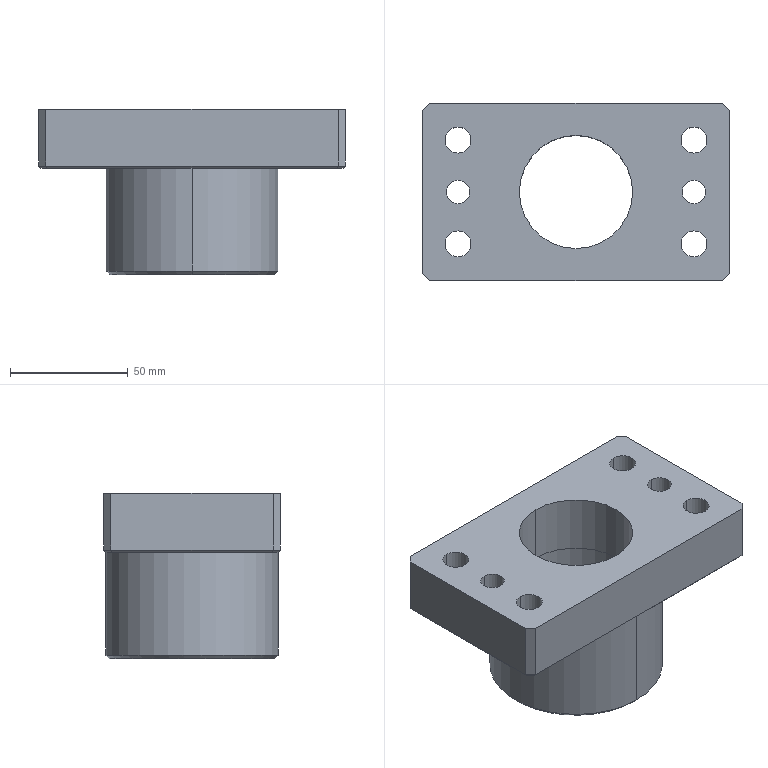Part | STEP file | PN_0058_id1506_x_t | 1 solid | 40 faces | box 130 x 75 x 70 mm | volume 291088 mm3 | plane 20 | cylinder 18 | cone 2 | commonest cylinder face diameters 11 x8 10 x4 48 x4 73 x2
STEP:
#1=CARTESIAN_POINT('',(-260.,-277.5,105.));
#2=VERTEX_POINT('',#1);
#3=CARTESIAN_POINT('',(-260.,-277.5,80.));
#4=VERTEX_POINT('',#3);
#5=CARTESIAN_POINT('',(-260.,-277.5,105.));
#6=DIRECTION('',(0.,0.,-1.));
#7=VECTOR('',#6,1.);
#8=LINE('',#5,#7);
#9=EDGE_CURVE('',#2,#4,#8,.T.);
#10=ORIENTED_EDGE('',*,*,#9,.F.);
#11=CARTESIAN_POINT('',(-260.,-266.5,105.));
#12=VERTEX_POINT('',#11);
#13=CARTESIAN_POINT('',(-260.,-272.,105.));
#14=DIRECTION('',(0.,0.,1.));
#15=DIRECTION('',(0.,-1.,0.));
#16=AXIS2_PLACEMENT_3D('',#13,#14,#15);
#17=CIRCLE('',#16,5.5);
#18=EDGE_CURVE('',#2,#12,#17,.T.);
#19=ORIENTED_EDGE('',*,*,#18,.T.);
#20=CARTESIAN_POINT('',(-260.,-266.5,80.));
#21=VERTEX_POINT('',#20);
#22=CARTESIAN_POINT('',(-260.,-266.5,105.));
#23=DIRECTION('',(0.,0.,1.));
#24=VECTOR('',#23,1.);
#25=LINE('',#22,#24);
#26=EDGE_CURVE('',#21,#12,#25,.T.);
#27=ORIENTED_EDGE('',*,*,#26,.F.);
#28=CARTESIAN_POINT('',(-260.,-272.,80.));
#29=DIRECTION('',(0.,0.,1.));
#30=DIRECTION('',(0.,-1.,0.));
#31=AXIS2_PLACEMENT_3D('',#28,#29,#30);
#32=CIRCLE('',#31,5.5);
#33=EDGE_CURVE('',#4,#21,#32,.T.);
#34=ORIENTED_EDGE('',*,*,#33,.F.);
#35=EDGE_LOOP('',(#10,#19,#27,#34));
#36=FACE_OUTER_BOUND('',#35,.T.);
#37=CARTESIAN_POINT('',(-260.,-272.,105.));
#38=DIRECTION('',(0.,0.,1.));
#39=DIRECTION('',(-1.,0.,0.));
#40=AXIS2_PLACEMENT_3D('',#37,#38,#39);
#41=CYLINDRICAL_SURFACE('',#40,5.5);
#42=ADVANCED_FACE('',(#36),#41,.F.);
#43=ORIENTED_EDGE('',*,*,#26,.T.);
#44=CARTESIAN_POINT('',(-260.,-272.,105.));
#45=DIRECTION('',(0.,0.,1.));
#46=DIRECTION('',(0.,1.,0.));
#47=AXIS2_PLACEMENT_3D('',#44,#45,#46);
#48=CIRCLE('',#47,5.5);
#49=EDGE_CURVE('',#12,#2,#48,.T.);
#50=ORIENTED_EDGE('',*,*,#49,.T.);
#51=ORIENTED_EDGE('',*,*,#9,.T.);
#52=CARTESIAN_POINT('',(-260.,-272.,80.));
#53=DIRECTION('',(0.,0.,1.));
#54=DIRECTION('',(0.,1.,0.));
#55=AXIS2_PLACEMENT_3D('',#52,#53,#54);
#56=CIRCLE('',#55,5.5);
#57=EDGE_CURVE('',#21,#4,#56,.T.);
#58=ORIENTED_EDGE('',*,*,#57,.F.);
#59=EDGE_LOOP('',(#43,#50,#51,#58));
#60=FACE_OUTER_BOUND('',#59,.T.);
#61=CARTESIAN_POINT('',(-260.,-272.,105.));
#62=DIRECTION('',(0.,0.,1.));
#63=DIRECTION('',(1.,0.,0.));
#64=AXIS2_PLACEMENT_3D('',#61,#62,#63);
#65=CYLINDRICAL_SURFACE('',#64,5.5);
#66=ADVANCED_FACE('',(#60),#65,.F.);
#67=CARTESIAN_POINT('',(-260.,-233.5,105.));
#68=VERTEX_POINT('',#67);
#69=CARTESIAN_POINT('',(-260.,-233.5,80.));
#70=VERTEX_POINT('',#69);
#71=CARTESIAN_POINT('',(-260.,-233.5,105.));
#72=DIRECTION('',(0.,0.,-1.));
#73=VECTOR('',#72,1.);
#74=LINE('',#71,#73);
#75=EDGE_CURVE('',#68,#70,#74,.T.);
#76=ORIENTED_EDGE('',*,*,#75,.F.);
#77=CARTESIAN_POINT('',(-260.,-222.5,105.));
#78=VERTEX_POINT('',#77);
#79=CARTESIAN_POINT('',(-260.,-228.,105.));
#80=DIRECTION('',(0.,0.,1.));
#81=DIRECTION('',(0.,-1.,0.));
#82=AXIS2_PLACEMENT_3D('',#79,#80,#81);
#83=CIRCLE('',#82,5.5);
#84=EDGE_CURVE('',#68,#78,#83,.T.);
#85=ORIENTED_EDGE('',*,*,#84,.T.);
#86=CARTESIAN_POINT('',(-260.,-222.5,80.));
#87=VERTEX_POINT('',#86);
#88=CARTESIAN_POINT('',(-260.,-222.5,105.));
#89=DIRECTION('',(0.,0.,1.));
#90=VECTOR('',#89,1.);
#91=LINE('',#88,#90);
#92=EDGE_CURVE('',#87,#78,#91,.T.);
#93=ORIENTED_EDGE('',*,*,#92,.F.);
#94=CARTESIAN_POINT('',(-260.,-228.,80.));
#95=DIRECTION('',(0.,0.,1.));
#96=DIRECTION('',(0.,-1.,0.));
#97=AXIS2_PLACEMENT_3D('',#94,#95,#96);
#98=CIRCLE('',#97,5.5);
#99=EDGE_CURVE('',#70,#87,#98,.T.);
#100=ORIENTED_EDGE('',*,*,#99,.F.);
#101=EDGE_LOOP('',(#76,#85,#93,#100));
#102=FACE_OUTER_BOUND('',#101,.T.);
#103=CARTESIAN_POINT('',(-260.,-228.,105.));
#104=DIRECTION('',(0.,0.,1.));
#105=DIRECTION('',(-1.,0.,0.));
#106=AXIS2_PLACEMENT_3D('',#103,#104,#105);
#107=CYLINDRICAL_SURFACE('',#106,5.5);
#108=ADVANCED_FACE('',(#102),#107,.F.);
#109=ORIENTED_EDGE('',*,*,#92,.T.);
#110=CARTESIAN_POINT('',(-260.,-228.,105.));
#111=DIRECTION('',(0.,0.,1.));
#112=DIRECTION('',(0.,1.,0.));
#113=AXIS2_PLACEMENT_3D('',#110,#111,#112);
#114=CIRCLE('',#113,5.5);
#115=EDGE_CURVE('',#78,#68,#114,.T.);
#116=ORIENTED_EDGE('',*,*,#115,.T.);
#117=ORIENTED_EDGE('',*,*,#75,.T.);
#118=CARTESIAN_POINT('',(-260.,-228.,80.));
#119=DIRECTION('',(0.,0.,1.));
#120=DIRECTION('',(0.,1.,0.));
#121=AXIS2_PLACEMENT_3D('',#118,#119,#120);
#122=CIRCLE('',#121,5.5);
#123=EDGE_CURVE('',#87,#70,#122,.T.);
#124=ORIENTED_EDGE('',*,*,#123,.F.);
#125=EDGE_LOOP('',(#109,#116,#117,#124));
#126=FACE_OUTER_BOUND('',#125,.T.);
#127=CARTESIAN_POINT('',(-260.,-228.,105.));
#128=DIRECTION('',(0.,0.,1.));
#129=DIRECTION('',(1.,0.,0.));
#130=AXIS2_PLACEMENT_3D('',#127,#128,#129);
#131=CYLINDRICAL_SURFACE('',#130,5.5);
#132=ADVANCED_FACE('',(#126),#131,.F.);
#133=CARTESIAN_POINT('',(-160.,-233.5,80.));
#134=VERTEX_POINT('',#133);
#135=CARTESIAN_POINT('',(-160.,-233.5,105.));
#136=VERTEX_POINT('',#135);
#137=CARTESIAN_POINT('',(-160.,-233.5,105.));
#138=DIRECTION('',(0.,0.,1.));
#139=VECTOR('',#138,1.);
#140=LINE('',#137,#139);
#141=EDGE_CURVE('',#134,#136,#140,.T.);
#142=ORIENTED_EDGE('',*,*,#141,.T.);
#143=CARTESIAN_POINT('',(-160.,-222.5,105.));
#144=VERTEX_POINT('',#143);
#145=CARTESIAN_POINT('',(-160.,-228.,105.));
#146=DIRECTION('',(0.,0.,1.));
#147=DIRECTION('',(0.,-1.,0.));
#148=AXIS2_PLACEMENT_3D('',#145,#146,#147);
#149=CIRCLE('',#148,5.5);
#150=EDGE_CURVE('',#136,#144,#149,.T.);
#151=ORIENTED_EDGE('',*,*,#150,.T.);
#152=CARTESIAN_POINT('',(-160.,-222.5,80.));
#153=VERTEX_POINT('',#152);
#154=CARTESIAN_POINT('',(-160.,-222.5,105.));
#155=DIRECTION('',(0.,0.,-1.));
#156=VECTOR('',#155,1.);
#157=LINE('',#154,#156);
#158=EDGE_CURVE('',#144,#153,#157,.T.);
#159=ORIENTED_EDGE('',*,*,#158,.T.);
#160=CARTESIAN_POINT('',(-160.,-228.,80.));
#161=DIRECTION('',(0.,0.,1.));
#162=DIRECTION('',(0.,-1.,0.));
#163=AXIS2_PLACEMENT_3D('',#160,#161,#162);
#164=CIRCLE('',#163,5.5);
#165=EDGE_CURVE('',#134,#153,#164,.T.);
#166=ORIENTED_EDGE('',*,*,#165,.F.);
#167=EDGE_LOOP('',(#142,#151,#159,#166));
#168=FACE_OUTER_BOUND('',#167,.T.);
#169=CARTESIAN_POINT('',(-160.,-228.,105.));
#170=DIRECTION('',(0.,0.,1.));
#171=DIRECTION('',(-1.,0.,0.));
#172=AXIS2_PLACEMENT_3D('',#169,#170,#171);
#173=CYLINDRICAL_SURFACE('',#172,5.5);
#174=ADVANCED_FACE('',(#168),#173,.F.);
#175=ORIENTED_EDGE('',*,*,#158,.F.);
#176=CARTESIAN_POINT('',(-160.,-228.,105.));
#177=DIRECTION('',(0.,0.,1.));
#178=DIRECTION('',(0.,1.,0.));
#179=AXIS2_PLACEMENT_3D('',#176,#177,#178);
#180=CIRCLE('',#179,5.5);
#181=EDGE_CURVE('',#144,#136,#180,.T.);
#182=ORIENTED_EDGE('',*,*,#181,.T.);
#183=ORIENTED_EDGE('',*,*,#141,.F.);
#184=CARTESIAN_POINT('',(-160.,-228.,80.));
#185=DIRECTION('',(0.,0.,1.));
#186=DIRECTION('',(0.,1.,0.));
#187=AXIS2_PLACEMENT_3D('',#184,#185,#186);
#188=CIRCLE('',#187,5.5);
#189=EDGE_CURVE('',#153,#134,#188,.T.);
#190=ORIENTED_EDGE('',*,*,#189,.F.);
#191=EDGE_LOOP('',(#175,#182,#183,#190));
#192=FACE_OUTER_BOUND('',#191,.T.);
#193=CARTESIAN_POINT('',(-160.,-228.,105.));
#194=DIRECTION('',(0.,0.,1.));
#195=DIRECTION('',(1.,0.,0.));
#196=AXIS2_PLACEMENT_3D('',#193,#194,#195);
#197=CYLINDRICAL_SURFACE('',#196,5.5);
#198=ADVANCED_FACE('',(#192),#197,.F.);
#199=CARTESIAN_POINT('',(-160.,-277.5,80.));
#200=VERTEX_POINT('',#199);
#201=CARTESIAN_POINT('',(-160.,-277.5,105.));
#202=VERTEX_POINT('',#201);
#203=CARTESIAN_POINT('',(-160.,-277.5,105.));
#204=DIRECTION('',(0.,0.,1.));
#205=VECTOR('',#204,1.);
#206=LINE('',#203,#205);
#207=EDGE_CURVE('',#200,#202,#206,.T.);
#208=ORIENTED_EDGE('',*,*,#207,.T.);
#209=CARTESIAN_POINT('',(-160.,-266.5,105.));
#210=VERTEX_POINT('',#209);
#211=CARTESIAN_POINT('',(-160.,-272.,105.));
#212=DIRECTION('',(0.,0.,1.));
#213=DIRECTION('',(0.,-1.,0.));
#214=AXIS2_PLACEMENT_3D('',#211,#212,#213);
#215=CIRCLE('',#214,5.5);
#216=EDGE_CURVE('',#202,#210,#215,.T.);
#217=ORIENTED_EDGE('',*,*,#216,.T.);
#218=CARTESIAN_POINT('',(-160.,-266.5,80.));
#219=VERTEX_POINT('',#218);
#220=CARTESIAN_POINT('',(-160.,-266.5,105.));
#221=DIRECTION('',(0.,0.,-1.));
#222=VECTOR('',#221,1.);
#223=LINE('',#220,#222);
#224=EDGE_CURVE('',#210,#219,#223,.T.);
#225=ORIENTED_EDGE('',*,*,#224,.T.);
#226=CARTESIAN_POINT('',(-160.,-272.,80.));
#227=DIRECTION('',(0.,0.,1.));
#228=DIRECTION('',(0.,-1.,0.));
#229=AXIS2_PLACEMENT_3D('',#226,#227,#228);
#230=CIRCLE('',#229,5.5);
#231=EDGE_CURVE('',#200,#219,#230,.T.);
#232=ORIENTED_EDGE('',*,*,#231,.F.);
#233=EDGE_LOOP('',(#208,#217,#225,#232));
#234=FACE_OUTER_BOUND('',#233,.T.);
#235=CARTESIAN_POINT('',(-160.,-272.,105.));
#236=DIRECTION('',(0.,0.,1.));
#237=DIRECTION('',(-1.,0.,0.));
#238=AXIS2_PLACEMENT_3D('',#235,#236,#237);
#239=CYLINDRICAL_SURFACE('',#238,5.5);
#240=ADVANCED_FACE('',(#234),#239,.F.);
#241=ORIENTED_EDGE('',*,*,#224,.F.);
#242=CARTESIAN_POINT('',(-160.,-272.,105.));
#243=DIRECTION('',(0.,0.,1.));
#244=DIRECTION('',(0.,1.,0.));
#245=AXIS2_PLACEMENT_3D('',#242,#243,#244);
#246=CIRCLE('',#245,5.5);
#247=EDGE_CURVE('',#210,#202,#246,.T.);
#248=ORIENTED_EDGE('',*,*,#247,.T.);
#249=ORIENTED_EDGE('',*,*,#207,.F.);
#250=CARTESIAN_POINT('',(-160.,-272.,80.));
#251=DIRECTION('',(0.,0.,1.));
#252=DIRECTION('',(0.,1.,0.));
#253=AXIS2_PLACEMENT_3D('',#250,#251,#252);
#254=CIRCLE('',#253,5.5);
#255=EDGE_CURVE('',#219,#200,#254,.T.);
#256=ORIENTED_EDGE('',*,*,#255,.F.);
#257=EDGE_LOOP('',(#241,#248,#249,#256));
#258=FACE_OUTER_BOUND('',#257,.T.);
#259=CARTESIAN_POINT('',(-160.,-272.,105.));
#260=DIRECTION('',(0.,0.,1.));
#261=DIRECTION('',(1.,0.,0.));
#262=AXIS2_PLACEMENT_3D('',#259,#260,#261);
#263=CYLINDRICAL_SURFACE('',#262,5.5);
#264=ADVANCED_FACE('',(#258),#263,.F.);
#265=CARTESIAN_POINT('',(-210.,-274.,105.));
#266=VERTEX_POINT('',#265);
#267=CARTESIAN_POINT('',(-210.,-274.,80.));
#268=VERTEX_POINT('',#267);
#269=CARTESIAN_POINT('',(-210.,-274.,105.));
#270=DIRECTION('',(0.,0.,-1.));
#271=VECTOR('',#270,1.);
#272=LINE('',#269,#271);
#273=EDGE_CURVE('',#266,#268,#272,.T.);
#274=ORIENTED_EDGE('',*,*,#273,.F.);
#275=CARTESIAN_POINT('',(-210.,-226.,105.));
#276=VERTEX_POINT('',#275);
#277=CARTESIAN_POINT('',(-210.,-250.,105.));
#278=DIRECTION('',(0.,0.,1.));
#279=DIRECTION('',(0.,-1.,0.));
#280=AXIS2_PLACEMENT_3D('',#277,#278,#279);
#281=CIRCLE('',#280,24.);
#282=EDGE_CURVE('',#266,#276,#281,.T.);
#283=ORIENTED_EDGE('',*,*,#282,.T.);
#284=CARTESIAN_POINT('',(-210.,-226.,80.));
#285=VERTEX_POINT('',#284);
#286=CARTESIAN_POINT('',(-210.,-226.,105.));
#287=DIRECTION('',(0.,0.,1.));
#288=VECTOR('',#287,1.);
#289=LINE('',#286,#288);
#290=EDGE_CURVE('',#285,#276,#289,.T.);
#291=ORIENTED_EDGE('',*,*,#290,.F.);
#292=CARTESIAN_POINT('',(-210.,-250.,80.));
#293=DIRECTION('',(0.,0.,1.));
#294=DIRECTION('',(0.,-1.,0.));
#295=AXIS2_PLACEMENT_3D('',#292,#293,#294);
#296=CIRCLE('',#295,24.);
#297=EDGE_CURVE('',#268,#285,#296,.T.);
#298=ORIENTED_EDGE('',*,*,#297,.F.);
#299=EDGE_LOOP('',(#274,#283,#291,#298));
#300=FACE_OUTER_BOUND('',#299,.T.);
#301=CARTESIAN_POINT('',(-210.,-250.,105.));
#302=DIRECTION('',(0.,0.,1.));
#303=DIRECTION('',(-1.,0.008727,0.));
#304=AXIS2_PLACEMENT_3D('',#301,#302,#303);
#305=CYLINDRICAL_SURFACE('',#304,24.);
#306=ADVANCED_FACE('',(#300),#305,.F.);
#307=ORIENTED_EDGE('',*,*,#290,.T.);
#308=CARTESIAN_POINT('',(-210.,-250.,105.));
#309=DIRECTION('',(0.,0.,1.));
#310=DIRECTION('',(0.,1.,0.));
#311=AXIS2_PLACEMENT_3D('',#308,#309,#310);
#312=CIRCLE('',#311,24.);
#313=EDGE_CURVE('',#276,#266,#312,.T.);
#314=ORIENTED_EDGE('',*,*,#313,.T.);
#315=ORIENTED_EDGE('',*,*,#273,.T.);
#316=CARTESIAN_POINT('',(-210.,-250.,80.));
#317=DIRECTION('',(0.,0.,1.));
#318=DIRECTION('',(0.,1.,0.));
#319=AXIS2_PLACEMENT_3D('',#316,#317,#318);
#320=CIRCLE('',#319,24.);
#321=EDGE_CURVE('',#285,#268,#320,.T.);
#322=ORIENTED_EDGE('',*,*,#321,.F.);
#323=EDGE_LOOP('',(#307,#314,#315,#322));
#324=FACE_OUTER_BOUND('',#323,.T.);
#325=CARTESIAN_POINT('',(-210.,-250.,105.));
#326=DIRECTION('',(0.,0.,1.));
#327=DIRECTION('',(1.,0.,0.));
#328=AXIS2_PLACEMENT_3D('',#325,#326,#327);
#329=CYLINDRICAL_SURFACE('',#328,24.);
#330=ADVANCED_FACE('',(#324),#329,.F.);
#331=ORIENTED_EDGE('',*,*,#297,.T.);
#332=CARTESIAN_POINT('',(-210.,-226.,35.));
#333=VERTEX_POINT('',#332);
#334=CARTESIAN_POINT('',(-210.,-226.,80.));
#335=DIRECTION('',(0.,0.,-1.));
#336=VECTOR('',#335,1.);
#337=LINE('',#334,#336);
#338=EDGE_CURVE('',#285,#333,#337,.T.);
#339=ORIENTED_EDGE('',*,*,#338,.T.);
#340=CARTESIAN_POINT('',(-210.,-274.,35.));
#341=VERTEX_POINT('',#340);
#342=CARTESIAN_POINT('',(-210.,-250.,35.));
#343=DIRECTION('',(0.,0.,1.));
#344=DIRECTION('',(0.,-1.,0.));
#345=AXIS2_PLACEMENT_3D('',#342,#343,#344);
#346=CIRCLE('',#345,24.);
#347=EDGE_CURVE('',#341,#333,#346,.T.);
#348=ORIENTED_EDGE('',*,*,#347,.F.);
#349=CARTESIAN_POINT('',(-210.,-274.,80.));
#350=DIRECTION('',(0.,0.,1.));
#351=VECTOR('',#350,1.);
#352=LINE('',#349,#351);
#353=EDGE_CURVE('',#341,#268,#352,.T.);
#354=ORIENTED_EDGE('',*,*,#353,.T.);
#355=EDGE_LOOP('',(#331,#339,#348,#354));
#356=FACE_OUTER_BOUND('',#355,.T.);
#357=CARTESIAN_POINT('',(-210.,-250.,105.));
#358=DIRECTION('',(0.,0.,1.));
#359=DIRECTION('',(-1.,0.008727,0.));
#360=AXIS2_PLACEMENT_3D('',#357,#358,#359);
#361=CYLINDRICAL_SURFACE('',#360,24.);
#362=ADVANCED_FACE('',(#356),#361,.F.);
#363=ORIENTED_EDGE('',*,*,#321,.T.);
#364=ORIENTED_EDGE('',*,*,#353,.F.);
#365=CARTESIAN_POINT('',(-210.,-250.,35.));
#366=DIRECTION('',(0.,0.,1.));
#367=DIRECTION('',(0.,1.,0.));
#368=AXIS2_PLACEMENT_3D('',#365,#366,#367);
#369=CIRCLE('',#368,24.);
#370=EDGE_CURVE('',#333,#341,#369,.T.);
#371=ORIENTED_EDGE('',*,*,#370,.F.);
#372=ORIENTED_EDGE('',*,*,#338,.F.);
#373=EDGE_LOOP('',(#363,#364,#371,#372));
#374=FACE_OUTER_BOUND('',#373,.T.);
#375=CARTESIAN_POINT('',(-210.,-250.,105.));
#376=DIRECTION('',(0.,0.,1.));
#377=DIRECTION('',(1.,0.,0.));
#378=AXIS2_PLACEMENT_3D('',#375,#376,#377);
#379=CYLINDRICAL_SURFACE('',#378,24.);
#380=ADVANCED_FACE('',(#374),#379,.F.);
#381=CARTESIAN_POINT('',(-260.,-245.,105.));
#382=VERTEX_POINT('',#381);
#383=CARTESIAN_POINT('',(-260.,-245.,80.));
#384=VERTEX_POINT('',#383);
#385=CARTESIAN_POINT('',(-260.,-245.,105.));
#386=DIRECTION('',(0.,0.,-1.));
#387=VECTOR('',#386,1.);
#388=LINE('',#385,#387);
#389=EDGE_CURVE('',#382,#384,#388,.T.);
#390=ORIENTED_EDGE('',*,*,#389,.F.);
#391=CARTESIAN_POINT('',(-260.,-255.,105.));
#392=VERTEX_POINT('',#391);
#393=CARTESIAN_POINT('',(-260.,-250.,105.));
#394=DIRECTION('',(0.,0.,1.));
#395=DIRECTION('',(0.,1.,0.));
#396=AXIS2_PLACEMENT_3D('',#393,#394,#395);
#397=CIRCLE('',#396,5.);
#398=EDGE_CURVE('',#382,#392,#397,.T.);
#399=ORIENTED_EDGE('',*,*,#398,.T.);
#400=CARTESIAN_POINT('',(-260.,-255.,80.));
#401=VERTEX_POINT('',#400);
#402=CARTESIAN_POINT('',(-260.,-255.,105.));
#403=DIRECTION('',(0.,0.,1.));
#404=VECTOR('',#403,1.);
#405=LINE('',#402,#404);
#406=EDGE_CURVE('',#401,#392,#405,.T.);
#407=ORIENTED_EDGE('',*,*,#406,.F.);
#408=CARTESIAN_POINT('',(-260.,-250.,80.));
#409=DIRECTION('',(0.,0.,-1.));
#410=DIRECTION('',(0.,-1.,0.));
#411=AXIS2_PLACEMENT_3D('',#408,#409,#410);
#412=CIRCLE('',#411,5.);
#413=EDGE_CURVE('',#401,#384,#412,.T.);
#414=ORIENTED_EDGE('',*,*,#413,.T.);
#415=EDGE_LOOP('',(#390,#399,#407,#414));
#416=FACE_OUTER_BOUND('',#415,.T.);
#417=CARTESIAN_POINT('',(-260.,-250.,105.));
#418=DIRECTION('',(0.,0.,1.));
#419=DIRECTION('',(1.,0.,0.));
#420=AXIS2_PLACEMENT_3D('',#417,#418,#419);
#421=CYLINDRICAL_SURFACE('',#420,5.);
#422=ADVANCED_FACE('',(#416),#421,.F.);
#423=ORIENTED_EDGE('',*,*,#389,.T.);
#424=CARTESIAN_POINT('',(-260.,-250.,80.));
#425=DIRECTION('',(0.,0.,-1.));
#426=DIRECTION('',(0.,1.,0.));
#427=AXIS2_PLACEMENT_3D('',#424,#425,#426);
#428=CIRCLE('',#427,5.);
#429=EDGE_CURVE('',#384,#401,#428,.T.);
#430=ORIENTED_EDGE('',*,*,#429,.T.);
#431=ORIENTED_EDGE('',*,*,#406,.T.);
#432=CARTESIAN_POINT('',(-260.,-250.,105.));
#433=DIRECTION('',(0.,0.,1.));
#434=DIRECTION('',(0.,-1.,0.));
#435=AXIS2_PLACEMENT_3D('',#432,#433,#434);
#436=CIRCLE('',#435,5.);
#437=EDGE_CURVE('',#392,#382,#436,.T.);
#438=ORIENTED_EDGE('',*,*,#437,.T.);
#439=EDGE_LOOP('',(#423,#430,#431,#438));
#440=FACE_OUTER_BOUND('',#439,.T.);
#441=CARTESIAN_POINT('',(-260.,-250.,105.));
#442=DIRECTION('',(0.,0.,1.));
#443=DIRECTION('',(-1.,0.,0.));
#444=AXIS2_PLACEMENT_3D('',#441,#442,#443);
#445=CYLINDRICAL_SURFACE('',#444,5.);
#446=ADVANCED_FACE('',(#440),#445,.F.);
#447=CARTESIAN_POINT('',(-160.,-245.,105.));
#448=VERTEX_POINT('',#447);
#449=CARTESIAN_POINT('',(-160.,-245.,80.));
#450=VERTEX_POINT('',#449);
#451=CARTESIAN_POINT('',(-160.,-245.,105.));
#452=DIRECTION('',(0.,0.,-1.));
#453=VECTOR('',#452,1.);
#454=LINE('',#451,#453);
#455=EDGE_CURVE('',#448,#450,#454,.T.);
#456=ORIENTED_EDGE('',*,*,#455,.F.);
#457=CARTESIAN_POINT('',(-160.,-255.,105.));
#458=VERTEX_POINT('',#457);
#459=CARTESIAN_POINT('',(-160.,-250.,105.));
#460=DIRECTION('',(0.,0.,1.));
#461=DIRECTION('',(0.,1.,0.));
#462=AXIS2_PLACEMENT_3D('',#459,#460,#461);
#463=CIRCLE('',#462,5.);
#464=EDGE_CURVE('',#448,#458,#463,.T.);
#465=ORIENTED_EDGE('',*,*,#464,.T.);
#466=CARTESIAN_POINT('',(-160.,-255.,80.));
#467=VERTEX_POINT('',#466);
#468=CARTESIAN_POINT('',(-160.,-255.,105.));
#469=DIRECTION('',(0.,0.,1.));
#470=VECTOR('',#469,1.);
#471=LINE('',#468,#470);
#472=EDGE_CURVE('',#467,#458,#471,.T.);
#473=ORIENTED_EDGE('',*,*,#472,.F.);
#474=CARTESIAN_POINT('',(-160.,-250.,80.));
#475=DIRECTION('',(0.,0.,-1.));
#476=DIRECTION('',(0.,-1.,0.));
#477=AXIS2_PLACEMENT_3D('',#474,#475,#476);
#478=CIRCLE('',#477,5.);
#479=EDGE_CURVE('',#467,#450,#478,.T.);
#480=ORIENTED_EDGE('',*,*,#479,.T.);
#481=EDGE_LOOP('',(#456,#465,#473,#480));
#482=FACE_OUTER_BOUND('',#481,.T.);
#483=CARTESIAN_POINT('',(-160.,-250.,105.));
#484=DIRECTION('',(0.,0.,1.));
#485=DIRECTION('',(1.,0.,0.));
#486=AXIS2_PLACEMENT_3D('',#483,#484,#485);
#487=CYLINDRICAL_SURFACE('',#486,5.);
#488=ADVANCED_FACE('',(#482),#487,.F.);
#489=ORIENTED_EDGE('',*,*,#455,.T.);
#490=CARTESIAN_POINT('',(-160.,-250.,80.));
#491=DIRECTION('',(0.,0.,-1.));
#492=DIRECTION('',(0.,1.,0.));
#493=AXIS2_PLACEMENT_3D('',#490,#491,#492);
#494=CIRCLE('',#493,5.);
#495=EDGE_CURVE('',#450,#467,#494,.T.);
#496=ORIENTED_EDGE('',*,*,#495,.T.);
#497=ORIENTED_EDGE('',*,*,#472,.T.);
#498=CARTESIAN_POINT('',(-160.,-250.,105.));
#499=DIRECTION('',(0.,0.,1.));
#500=DIRECTION('',(0.,-1.,0.));
#501=AXIS2_PLACEMENT_3D('',#498,#499,#500);
#502=CIRCLE('',#501,5.);
#503=EDGE_CURVE('',#458,#448,#502,.T.);
#504=ORIENTED_EDGE('',*,*,#503,.T.);
#505=EDGE_LOOP('',(#489,#496,#497,#504));
#506=FACE_OUTER_BOUND('',#505,.T.);
#507=CARTESIAN_POINT('',(-160.,-250.,105.));
#508=DIRECTION('',(0.,0.,1.));
#509=DIRECTION('',(-1.,0.,0.));
#510=AXIS2_PLACEMENT_3D('',#507,#508,#509);
#511=CYLINDRICAL_SURFACE('',#510,5.);
#512=ADVANCED_FACE('',(#506),#511,.F.);
#513=CARTESIAN_POINT('',(-148.,-212.5,105.));
#514=VERTEX_POINT('',#513);
#515=CARTESIAN_POINT('',(-145.,-215.5,105.));
#516=VERTEX_POINT('',#515);
#517=CARTESIAN_POINT('',(-148.,-212.5,105.));
#518=DIRECTION('',(0.7071,-0.7071,0.));
#519=VECTOR('',#518,1.);
#520=LINE('',#517,#519);
#521=EDGE_CURVE('',#514,#516,#520,.T.);
#522=ORIENTED_EDGE('',*,*,#521,.F.);
#523=CARTESIAN_POINT('',(-272.,-212.5,105.));
#524=VERTEX_POINT('',#523);
#525=CARTESIAN_POINT('',(-272.,-212.5,105.));
#526=DIRECTION('',(1.,0.,0.));
#527=VECTOR('',#526,1.);
#528=LINE('',#525,#527);
#529=EDGE_CURVE('',#524,#514,#528,.T.);
#530=ORIENTED_EDGE('',*,*,#529,.F.);
#531=CARTESIAN_POINT('',(-275.,-215.5,105.));
#532=VERTEX_POINT('',#531);
#533=CARTESIAN_POINT('',(-275.,-215.5,105.));
#534=DIRECTION('',(0.7071,0.7071,0.));
#535=VECTOR('',#534,1.);
#536=LINE('',#533,#535);
#537=EDGE_CURVE('',#532,#524,#536,.T.);
#538=ORIENTED_EDGE('',*,*,#537,.F.);
#539=CARTESIAN_POINT('',(-275.,-284.5,105.));
#540=VERTEX_POINT('',#539);
#541=CARTESIAN_POINT('',(-275.,-284.5,105.));
#542=DIRECTION('',(0.,1.,0.));
#543=VECTOR('',#542,1.);
#544=LINE('',#541,#543);
#545=EDGE_CURVE('',#540,#532,#544,.T.);
#546=ORIENTED_EDGE('',*,*,#545,.F.);
#547=CARTESIAN_POINT('',(-272.,-287.5,105.));
#548=VERTEX_POINT('',#547);
#549=CARTESIAN_POINT('',(-272.,-287.5,105.));
#550=DIRECTION('',(-0.7071,0.7071,0.));
#551=VECTOR('',#550,1.);
#552=LINE('',#549,#551);
#553=EDGE_CURVE('',#548,#540,#552,.T.);
#554=ORIENTED_EDGE('',*,*,#553,.F.);
#555=CARTESIAN_POINT('',(-148.,-287.5,105.));
#556=VERTEX_POINT('',#555);
#557=CARTESIAN_POINT('',(-148.,-287.5,105.));
#558=DIRECTION('',(-1.,0.,0.));
#559=VECTOR('',#558,1.);
#560=LINE('',#557,#559);
#561=EDGE_CURVE('',#556,#548,#560,.T.);
#562=ORIENTED_EDGE('',*,*,#561,.F.);
#563=CARTESIAN_POINT('',(-145.,-284.5,105.));
#564=VERTEX_POINT('',#563);
#565=CARTESIAN_POINT('',(-145.,-284.5,105.));
#566=DIRECTION('',(-0.7071,-0.7071,0.));
#567=VECTOR('',#566,1.);
#568=LINE('',#565,#567);
#569=EDGE_CURVE('',#564,#556,#568,.T.);
#570=ORIENTED_EDGE('',*,*,#569,.F.);
#571=CARTESIAN_POINT('',(-145.,-215.5,105.));
#572=DIRECTION('',(0.,-1.,0.));
#573=VECTOR('',#572,1.);
#574=LINE('',#571,#573);
#575=EDGE_CURVE('',#516,#564,#574,.T.);
#576=ORIENTED_EDGE('',*,*,#575,.F.);
#577=EDGE_LOOP('',(#522,#530,#538,#546,#554,#562,#570,#576));
#578=FACE_BOUND('',#577,.T.);
#579=ORIENTED_EDGE('',*,*,#503,.F.);
#580=ORIENTED_EDGE('',*,*,#464,.F.);
#581=EDGE_LOOP('',(#579,#580));
#582=FACE_BOUND('',#581,.T.);
#583=ORIENTED_EDGE('',*,*,#437,.F.);
#584=ORIENTED_EDGE('',*,*,#398,.F.);
#585=EDGE_LOOP('',(#583,#584));
#586=FACE_BOUND('',#585,.T.);
#587=ORIENTED_EDGE('',*,*,#18,.F.);
#588=ORIENTED_EDGE('',*,*,#49,.F.);
#589=EDGE_LOOP('',(#587,#588));
#590=FACE_BOUND('',#589,.T.);
#591=ORIENTED_EDGE('',*,*,#84,.F.);
#592=ORIENTED_EDGE('',*,*,#115,.F.);
#593=EDGE_LOOP('',(#591,#592));
#594=FACE_BOUND('',#593,.T.);
#595=ORIENTED_EDGE('',*,*,#150,.F.);
#596=ORIENTED_EDGE('',*,*,#181,.F.);
#597=EDGE_LOOP('',(#595,#596));
#598=FACE_BOUND('',#597,.T.);
#599=ORIENTED_EDGE('',*,*,#216,.F.);
#600=ORIENTED_EDGE('',*,*,#247,.F.);
#601=EDGE_LOOP('',(#599,#600));
#602=FACE_BOUND('',#601,.T.);
#603=ORIENTED_EDGE('',*,*,#282,.F.);
#604=ORIENTED_EDGE('',*,*,#313,.F.);
#605=EDGE_LOOP('',(#603,#604));
#606=FACE_BOUND('',#605,.T.);
#607=CARTESIAN_POINT('',(-285.,-295.,105.));
#608=DIRECTION('',(0.,0.,1.));
#609=DIRECTION('',(1.,0.,0.));
#610=AXIS2_PLACEMENT_3D('',#607,#608,#609);
#611=PLANE('',#610);
#612=ADVANCED_FACE('',(#578,#582,#586,#590,#594,#598,#602,#606),#611,.T.);
#613=CARTESIAN_POINT('',(-210.,-286.5,36.5));
#614=VERTEX_POINT('',#613);
#615=CARTESIAN_POINT('',(-210.,-213.5,36.5));
#616=VERTEX_POINT('',#615);
#617=CARTESIAN_POINT('',(-210.,-250.,36.5));
#618=DIRECTION('',(0.,0.,-1.));
#619=DIRECTION('',(0.,-1.,0.));
#620=AXIS2_PLACEMENT_3D('',#617,#618,#619);
#621=CIRCLE('',#620,36.5);
#622=EDGE_CURVE('',#614,#616,#621,.T.);
#623=ORIENTED_EDGE('',*,*,#622,.F.);
#624=CARTESIAN_POINT('',(-210.,-286.5,80.));
#625=VERTEX_POINT('',#624);
#626=CARTESIAN_POINT('',(-210.,-286.5,80.));
#627=DIRECTION('',(0.,0.,1.));
#628=VECTOR('',#627,1.);
#629=LINE('',#626,#628);
#630=EDGE_CURVE('',#614,#625,#629,.T.);
#631=ORIENTED_EDGE('',*,*,#630,.T.);
#632=CARTESIAN_POINT('',(-210.,-213.5,80.));
#633=VERTEX_POINT('',#632);
#634=CARTESIAN_POINT('',(-210.,-250.,80.));
#635=DIRECTION('',(0.,0.,-1.));
#636=DIRECTION('',(0.,-1.,0.));
#637=AXIS2_PLACEMENT_3D('',#634,#635,#636);
#638=CIRCLE('',#637,36.5);
#639=EDGE_CURVE('',#625,#633,#638,.T.);
#640=ORIENTED_EDGE('',*,*,#639,.T.);
#641=CARTESIAN_POINT('',(-210.,-213.5,80.));
#642=DIRECTION('',(0.,0.,-1.));
#643=VECTOR('',#642,1.);
#644=LINE('',#641,#643);
#645=EDGE_CURVE('',#633,#616,#644,.T.);
#646=ORIENTED_EDGE('',*,*,#645,.T.);
#647=EDGE_LOOP('',(#623,#631,#640,#646));
#648=FACE_OUTER_BOUND('',#647,.T.);
#649=CARTESIAN_POINT('',(-210.,-250.,105.));
#650=DIRECTION('',(0.,0.,1.));
#651=DIRECTION('',(1.,0.,0.));
#652=AXIS2_PLACEMENT_3D('',#649,#650,#651);
#653=CYLINDRICAL_SURFACE('',#652,36.5);
#654=ADVANCED_FACE('',(#648),#653,.T.);
#655=CARTESIAN_POINT('',(-210.,-250.,36.5));
#656=DIRECTION('',(0.,0.,-1.));
#657=DIRECTION('',(0.,1.,0.));
#658=AXIS2_PLACEMENT_3D('',#655,#656,#657);
#659=CIRCLE('',#658,36.5);
#660=EDGE_CURVE('',#616,#614,#659,.T.);
#661=ORIENTED_EDGE('',*,*,#660,.F.);
#662=ORIENTED_EDGE('',*,*,#645,.F.);
#663=CARTESIAN_POINT('',(-210.,-250.,80.));
#664=DIRECTION('',(0.,0.,-1.));
#665=DIRECTION('',(0.,1.,0.));
#666=AXIS2_PLACEMENT_3D('',#663,#664,#665);
#667=CIRCLE('',#666,36.5);
#668=EDGE_CURVE('',#633,#625,#667,.T.);
#669=ORIENTED_EDGE('',*,*,#668,.T.);
#670=ORIENTED_EDGE('',*,*,#630,.F.);
#671=EDGE_LOOP('',(#661,#662,#669,#670));
#672=FACE_OUTER_BOUND('',#671,.T.);
#673=CARTESIAN_POINT('',(-210.,-250.,105.));
#674=DIRECTION('',(0.,0.,1.));
#675=DIRECTION('',(-1.,0.,0.));
#676=AXIS2_PLACEMENT_3D('',#673,#674,#675);
#677=CYLINDRICAL_SURFACE('',#676,36.5);
#678=ADVANCED_FACE('',(#672),#677,.T.);
#679=CARTESIAN_POINT('',(-210.,-215.,35.));
#680=VERTEX_POINT('',#679);
#681=CARTESIAN_POINT('',(-210.,-285.,35.));
#682=VERTEX_POINT('',#681);
#683=CARTESIAN_POINT('',(-210.,-250.,35.));
#684=DIRECTION('',(0.,0.,1.));
#685=DIRECTION('',(0.,1.,0.));
#686=AXIS2_PLACEMENT_3D('',#683,#684,#685);
#687=CIRCLE('',#686,35.);
#688=EDGE_CURVE('',#680,#682,#687,.T.);
#689=ORIENTED_EDGE('',*,*,#688,.F.);
#690=CARTESIAN_POINT('',(-210.,-250.,35.));
#691=DIRECTION('',(0.,0.,1.));
#692=DIRECTION('',(0.,-1.,0.));
#693=AXIS2_PLACEMENT_3D('',#690,#691,#692);
#694=CIRCLE('',#693,35.);
#695=EDGE_CURVE('',#682,#680,#694,.T.);
#696=ORIENTED_EDGE('',*,*,#695,.F.);
#697=EDGE_LOOP('',(#689,#696));
#698=FACE_BOUND('',#697,.T.);
#699=ORIENTED_EDGE('',*,*,#347,.T.);
#700=ORIENTED_EDGE('',*,*,#370,.T.);
#701=EDGE_LOOP('',(#699,#700));
#702=FACE_BOUND('',#701,.T.);
#703=CARTESIAN_POINT('',(-168.,-208.,35.));
#704=DIRECTION('',(0.,0.,-1.));
#705=DIRECTION('',(0.,-1.,0.));
#706=AXIS2_PLACEMENT_3D('',#703,#704,#705);
#707=PLANE('',#706);
#708=ADVANCED_FACE('',(#698,#702),#707,.T.);
#709=CARTESIAN_POINT('',(-210.,-213.5,36.5));
#710=DIRECTION('',(0.,0.7071,0.7071));
#711=VECTOR('',#710,1.);
#712=LINE('',#709,#711);
#713=EDGE_CURVE('',#680,#616,#712,.T.);
#714=ORIENTED_EDGE('',*,*,#713,.F.);
#715=ORIENTED_EDGE('',*,*,#688,.T.);
#716=CARTESIAN_POINT('',(-210.,-286.5,36.5));
#717=DIRECTION('',(0.,0.7071,-0.7071));
#718=VECTOR('',#717,1.);
#719=LINE('',#716,#718);
#720=EDGE_CURVE('',#614,#682,#719,.T.);
#721=ORIENTED_EDGE('',*,*,#720,.F.);
#722=ORIENTED_EDGE('',*,*,#622,.T.);
#723=EDGE_LOOP('',(#714,#715,#721,#722));
#724=FACE_OUTER_BOUND('',#723,.T.);
#725=CARTESIAN_POINT('',(-210.,-250.,36.5));
#726=DIRECTION('',(0.,0.,1.));
#727=DIRECTION('',(0.9998,0.01745,0.));
#728=AXIS2_PLACEMENT_3D('',#725,#726,#727);
#729=CONICAL_SURFACE('',#728,36.5,45.);
#730=ADVANCED_FACE('',(#724),#729,.T.);
#731=ORIENTED_EDGE('',*,*,#713,.T.);
#732=ORIENTED_EDGE('',*,*,#660,.T.);
#733=ORIENTED_EDGE('',*,*,#720,.T.);
#734=ORIENTED_EDGE('',*,*,#695,.T.);
#735=EDGE_LOOP('',(#731,#732,#733,#734));
#736=FACE_OUTER_BOUND('',#735,.T.);
#737=CARTESIAN_POINT('',(-210.,-250.,36.5));
#738=DIRECTION('',(0.,0.,1.));
#739=DIRECTION('',(-1.,0.,0.));
#740=AXIS2_PLACEMENT_3D('',#737,#738,#739);
#741=CONICAL_SURFACE('',#740,36.5,45.);
#742=ADVANCED_FACE('',(#736),#741,.T.);
#743=CARTESIAN_POINT('',(-272.,-287.5,81.));
#744=VERTEX_POINT('',#743);
#745=CARTESIAN_POINT('',(-275.,-284.5,81.));
#746=VERTEX_POINT('',#745);
#747=CARTESIAN_POINT('',(-272.,-287.5,81.));
#748=DIRECTION('',(-0.7071,0.7071,0.));
#749=VECTOR('',#748,1.);
#750=LINE('',#747,#749);
#751=EDGE_CURVE('',#744,#746,#750,.T.);
#752=ORIENTED_EDGE('',*,*,#751,.F.);
#753=CARTESIAN_POINT('',(-272.,-287.5,81.));
#754=DIRECTION('',(0.,0.,1.));
#755=VECTOR('',#754,1.);
#756=LINE('',#753,#755);
#757=EDGE_CURVE('',#744,#548,#756,.T.);
#758=ORIENTED_EDGE('',*,*,#757,.T.);
#759=ORIENTED_EDGE('',*,*,#553,.T.);
#760=CARTESIAN_POINT('',(-275.,-284.5,105.));
#761=DIRECTION('',(0.,0.,-1.));
#762=VECTOR('',#761,1.);
#763=LINE('',#760,#762);
#764=EDGE_CURVE('',#540,#746,#763,.T.);
#765=ORIENTED_EDGE('',*,*,#764,.T.);
#766=EDGE_LOOP('',(#752,#758,#759,#765));
#767=FACE_OUTER_BOUND('',#766,.T.);
#768=CARTESIAN_POINT('',(-271.7,-287.8,107.4));
#769=DIRECTION('',(-0.7071,-0.7071,0.));
#770=DIRECTION('',(-0.7071,0.7071,0.));
#771=AXIS2_PLACEMENT_3D('',#768,#769,#770);
#772=PLANE('',#771);
#773=ADVANCED_FACE('',(#767),#772,.T.);
#774=CARTESIAN_POINT('',(-275.,-215.5,81.));
#775=VERTEX_POINT('',#774);
#776=CARTESIAN_POINT('',(-272.,-212.5,81.));
#777=VERTEX_POINT('',#776);
#778=CARTESIAN_POINT('',(-275.,-215.5,81.));
#779=DIRECTION('',(0.7071,0.7071,0.));
#780=VECTOR('',#779,1.);
#781=LINE('',#778,#780);
#782=EDGE_CURVE('',#775,#777,#781,.T.);
#783=ORIENTED_EDGE('',*,*,#782,.F.);
#784=CARTESIAN_POINT('',(-275.,-215.5,81.));
#785=DIRECTION('',(0.,0.,1.));
#786=VECTOR('',#785,1.);
#787=LINE('',#784,#786);
#788=EDGE_CURVE('',#775,#532,#787,.T.);
#789=ORIENTED_EDGE('',*,*,#788,.T.);
#790=ORIENTED_EDGE('',*,*,#537,.T.);
#791=CARTESIAN_POINT('',(-272.,-212.5,105.));
#792=DIRECTION('',(0.,0.,-1.));
#793=VECTOR('',#792,1.);
#794=LINE('',#791,#793);
#795=EDGE_CURVE('',#524,#777,#794,.T.);
#796=ORIENTED_EDGE('',*,*,#795,.T.);
#797=EDGE_LOOP('',(#783,#789,#790,#796));
#798=FACE_OUTER_BOUND('',#797,.T.);
#799=CARTESIAN_POINT('',(-275.3,-215.8,78.6));
#800=DIRECTION('',(-0.7071,0.7071,0.));
#801=DIRECTION('',(0.,0.,1.));
#802=AXIS2_PLACEMENT_3D('',#799,#800,#801);
#803=PLANE('',#802);
#804=ADVANCED_FACE('',(#798),#803,.T.);
#805=CARTESIAN_POINT('',(-148.,-212.5,81.));
#806=VERTEX_POINT('',#805);
#807=CARTESIAN_POINT('',(-145.,-215.5,81.));
#808=VERTEX_POINT('',#807);
#809=CARTESIAN_POINT('',(-148.,-212.5,81.));
#810=DIRECTION('',(0.7071,-0.7071,0.));
#811=VECTOR('',#810,1.);
#812=LINE('',#809,#811);
#813=EDGE_CURVE('',#806,#808,#812,.T.);
#814=ORIENTED_EDGE('',*,*,#813,.F.);
#815=CARTESIAN_POINT('',(-148.,-212.5,81.));
#816=DIRECTION('',(0.,0.,1.));
#817=VECTOR('',#816,1.);
#818=LINE('',#815,#817);
#819=EDGE_CURVE('',#806,#514,#818,.T.);
#820=ORIENTED_EDGE('',*,*,#819,.T.);
#821=ORIENTED_EDGE('',*,*,#521,.T.);
#822=CARTESIAN_POINT('',(-145.,-215.5,105.));
#823=DIRECTION('',(0.,0.,-1.));
#824=VECTOR('',#823,1.);
#825=LINE('',#822,#824);
#826=EDGE_CURVE('',#516,#808,#825,.T.);
#827=ORIENTED_EDGE('',*,*,#826,.T.);
#828=EDGE_LOOP('',(#814,#820,#821,#827));
#829=FACE_OUTER_BOUND('',#828,.T.);
#830=CARTESIAN_POINT('',(-144.7,-215.8,107.4));
#831=DIRECTION('',(0.7071,0.7071,0.));
#832=DIRECTION('',(0.,0.,-1.));
#833=AXIS2_PLACEMENT_3D('',#830,#831,#832);
#834=PLANE('',#833);
#835=ADVANCED_FACE('',(#829),#834,.T.);
#836=CARTESIAN_POINT('',(-145.,-284.5,81.));
#837=VERTEX_POINT('',#836);
#838=CARTESIAN_POINT('',(-148.,-287.5,81.));
#839=VERTEX_POINT('',#838);
#840=CARTESIAN_POINT('',(-145.,-284.5,81.));
#841=DIRECTION('',(-0.7071,-0.7071,0.));
#842=VECTOR('',#841,1.);
#843=LINE('',#840,#842);
#844=EDGE_CURVE('',#837,#839,#843,.T.);
#845=ORIENTED_EDGE('',*,*,#844,.F.);
#846=CARTESIAN_POINT('',(-145.,-284.5,81.));
#847=DIRECTION('',(0.,0.,1.));
#848=VECTOR('',#847,1.);
#849=LINE('',#846,#848);
#850=EDGE_CURVE('',#837,#564,#849,.T.);
#851=ORIENTED_EDGE('',*,*,#850,.T.);
#852=ORIENTED_EDGE('',*,*,#569,.T.);
#853=CARTESIAN_POINT('',(-148.,-287.5,105.));
#854=DIRECTION('',(0.,0.,-1.));
#855=VECTOR('',#854,1.);
#856=LINE('',#853,#855);
#857=EDGE_CURVE('',#556,#839,#856,.T.);
#858=ORIENTED_EDGE('',*,*,#857,.T.);
#859=EDGE_LOOP('',(#845,#851,#852,#858));
#860=FACE_OUTER_BOUND('',#859,.T.);
#861=CARTESIAN_POINT('',(-148.3,-287.8,107.4));
#862=DIRECTION('',(0.7071,-0.7071,0.));
#863=DIRECTION('',(0.,0.,-1.));
#864=AXIS2_PLACEMENT_3D('',#861,#862,#863);
#865=PLANE('',#864);
#866=ADVANCED_FACE('',(#860),#865,.T.);
#867=CARTESIAN_POINT('',(-145.,-215.5,81.));
#868=DIRECTION('',(0.,-1.,0.));
#869=VECTOR('',#868,1.);
#870=LINE('',#867,#869);
#871=EDGE_CURVE('',#808,#837,#870,.T.);
#872=ORIENTED_EDGE('',*,*,#871,.F.);
#873=ORIENTED_EDGE('',*,*,#826,.F.);
#874=ORIENTED_EDGE('',*,*,#575,.T.);
#875=ORIENTED_EDGE('',*,*,#850,.F.);
#876=EDGE_LOOP('',(#872,#873,#874,#875));
#877=FACE_OUTER_BOUND('',#876,.T.);
#878=CARTESIAN_POINT('',(-145.,-291.4,78.6));
#879=DIRECTION('',(1.,0.,0.));
#880=DIRECTION('',(0.,1.,0.));
#881=AXIS2_PLACEMENT_3D('',#878,#879,#880);
#882=PLANE('',#881);
#883=ADVANCED_FACE('',(#877),#882,.T.);
#884=CARTESIAN_POINT('',(-146.,-215.914,80.));
#885=VERTEX_POINT('',#884);
#886=CARTESIAN_POINT('',(-146.,-215.914,80.));
#887=DIRECTION('',(0.6786,0.2811,0.6786));
#888=VECTOR('',#887,1.);
#889=LINE('',#886,#888);
#890=EDGE_CURVE('',#885,#808,#889,.T.);
#891=ORIENTED_EDGE('',*,*,#890,.T.);
#892=ORIENTED_EDGE('',*,*,#871,.T.);
#893=CARTESIAN_POINT('',(-146.,-284.086,80.));
#894=VERTEX_POINT('',#893);
#895=CARTESIAN_POINT('',(-145.,-284.5,81.));
#896=DIRECTION('',(-0.6786,0.2811,-0.6786));
#897=VECTOR('',#896,1.);
#898=LINE('',#895,#897);
#899=EDGE_CURVE('',#837,#894,#898,.T.);
#900=ORIENTED_EDGE('',*,*,#899,.T.);
#901=CARTESIAN_POINT('',(-146.,-284.086,80.));
#902=DIRECTION('',(0.,1.,0.));
#903=VECTOR('',#902,1.);
#904=LINE('',#901,#903);
#905=EDGE_CURVE('',#894,#885,#904,.T.);
#906=ORIENTED_EDGE('',*,*,#905,.T.);
#907=EDGE_LOOP('',(#891,#892,#900,#906));
#908=FACE_OUTER_BOUND('',#907,.T.);
#909=CARTESIAN_POINT('',(-144.9,-208.6,81.1));
#910=DIRECTION('',(0.7071,0.,-0.7071));
#911=DIRECTION('',(0.,-1.,0.));
#912=AXIS2_PLACEMENT_3D('',#909,#910,#911);
#913=PLANE('',#912);
#914=ADVANCED_FACE('',(#908),#913,.T.);
#915=CARTESIAN_POINT('',(-148.414,-213.5,80.));
#916=VERTEX_POINT('',#915);
#917=CARTESIAN_POINT('',(-148.,-212.5,81.));
#918=DIRECTION('',(-0.2811,-0.6786,-0.6786));
#919=VECTOR('',#918,1.);
#920=LINE('',#917,#919);
#921=EDGE_CURVE('',#806,#916,#920,.T.);
#922=ORIENTED_EDGE('',*,*,#921,.F.);
#923=ORIENTED_EDGE('',*,*,#813,.T.);
#924=ORIENTED_EDGE('',*,*,#890,.F.);
#925=CARTESIAN_POINT('',(-146.,-215.914,80.));
#926=DIRECTION('',(-0.7071,0.7071,0.));
#927=VECTOR('',#926,1.);
#928=LINE('',#925,#927);
#929=EDGE_CURVE('',#885,#916,#928,.T.);
#930=ORIENTED_EDGE('',*,*,#929,.T.);
#931=EDGE_LOOP('',(#922,#923,#924,#930));
#932=FACE_OUTER_BOUND('',#931,.T.);
#933=CARTESIAN_POINT('',(-144.659,-213.339,82.769));
#934=DIRECTION('',(0.5,0.5,-0.7071));
#935=DIRECTION('',(0.,-0.8165,-0.5774));
#936=AXIS2_PLACEMENT_3D('',#933,#934,#935);
#937=PLANE('',#936);
#938=ADVANCED_FACE('',(#932),#937,.T.);
#939=CARTESIAN_POINT('',(-272.,-212.5,81.));
#940=DIRECTION('',(1.,0.,0.));
#941=VECTOR('',#940,1.);
#942=LINE('',#939,#941);
#943=EDGE_CURVE('',#777,#806,#942,.T.);
#944=ORIENTED_EDGE('',*,*,#943,.F.);
#945=ORIENTED_EDGE('',*,*,#795,.F.);
#946=ORIENTED_EDGE('',*,*,#529,.T.);
#947=ORIENTED_EDGE('',*,*,#819,.F.);
#948=EDGE_LOOP('',(#944,#945,#946,#947));
#949=FACE_OUTER_BOUND('',#948,.T.);
#950=CARTESIAN_POINT('',(-282.,-212.5,107.4));
#951=DIRECTION('',(0.,1.,0.));
#952=DIRECTION('',(1.,0.,0.));
#953=AXIS2_PLACEMENT_3D('',#950,#951,#952);
#954=PLANE('',#953);
#955=ADVANCED_FACE('',(#949),#954,.T.);
#956=CARTESIAN_POINT('',(-271.586,-213.5,80.));
#957=VERTEX_POINT('',#956);
#958=CARTESIAN_POINT('',(-271.586,-213.5,80.));
#959=DIRECTION('',(-0.2811,0.6786,0.6786));
#960=VECTOR('',#959,1.);
#961=LINE('',#958,#960);
#962=EDGE_CURVE('',#957,#777,#961,.T.);
#963=ORIENTED_EDGE('',*,*,#962,.T.);
#964=ORIENTED_EDGE('',*,*,#943,.T.);
#965=ORIENTED_EDGE('',*,*,#921,.T.);
#966=CARTESIAN_POINT('',(-148.414,-213.5,80.));
#967=DIRECTION('',(-1.,0.,0.));
#968=VECTOR('',#967,1.);
#969=LINE('',#966,#968);
#970=EDGE_CURVE('',#916,#633,#969,.T.);
#971=ORIENTED_EDGE('',*,*,#970,.T.);
#972=CARTESIAN_POINT('',(-210.,-213.5,80.));
#973=DIRECTION('',(-1.,0.,0.));
#974=VECTOR('',#973,1.);
#975=LINE('',#972,#974);
#976=EDGE_CURVE('',#633,#957,#975,.T.);
#977=ORIENTED_EDGE('',*,*,#976,.T.);
#978=EDGE_LOOP('',(#963,#964,#965,#971,#977));
#979=FACE_OUTER_BOUND('',#978,.T.);
#980=CARTESIAN_POINT('',(-138.,-213.6,79.9));
#981=DIRECTION('',(0.,0.7071,-0.7071));
#982=DIRECTION('',(-1.,0.,0.));
#983=AXIS2_PLACEMENT_3D('',#980,#981,#982);
#984=PLANE('',#983);
#985=ADVANCED_FACE('',(#979),#984,.T.);
#986=CARTESIAN_POINT('',(-274.,-215.914,80.));
#987=VERTEX_POINT('',#986);
#988=CARTESIAN_POINT('',(-275.,-215.5,81.));
#989=DIRECTION('',(0.6786,-0.2811,-0.6786));
#990=VECTOR('',#989,1.);
#991=LINE('',#988,#990);
#992=EDGE_CURVE('',#775,#987,#991,.T.);
#993=ORIENTED_EDGE('',*,*,#992,.F.);
#994=ORIENTED_EDGE('',*,*,#782,.T.);
#995=ORIENTED_EDGE('',*,*,#962,.F.);
#996=CARTESIAN_POINT('',(-271.586,-213.5,80.));
#997=DIRECTION('',(-0.7071,-0.7071,0.));
#998=VECTOR('',#997,1.);
#999=LINE('',#996,#998);
#1000=EDGE_CURVE('',#957,#987,#999,.T.);
#1001=ORIENTED_EDGE('',*,*,#1000,.T.);
#1002=EDGE_LOOP('',(#993,#994,#995,#1001));
#1003=FACE_OUTER_BOUND('',#1002,.T.);
#1004=CARTESIAN_POINT('',(-272.23,-216.256,78.507));
#1005=DIRECTION('',(-0.5,0.5,-0.7071));
#1006=DIRECTION('',(-0.8165,0.,0.5774));
#1007=AXIS2_PLACEMENT_3D('',#1004,#1005,#1006);
#1008=PLANE('',#1007);
#1009=ADVANCED_FACE('',(#1003),#1008,.T.);
#1010=CARTESIAN_POINT('',(-275.,-284.5,81.));
#1011=DIRECTION('',(0.,1.,0.));
#1012=VECTOR('',#1011,1.);
#1013=LINE('',#1010,#1012);
#1014=EDGE_CURVE('',#746,#775,#1013,.T.);
#1015=ORIENTED_EDGE('',*,*,#1014,.F.);
#1016=ORIENTED_EDGE('',*,*,#764,.F.);
#1017=ORIENTED_EDGE('',*,*,#545,.T.);
#1018=ORIENTED_EDGE('',*,*,#788,.F.);
#1019=EDGE_LOOP('',(#1015,#1016,#1017,#1018));
#1020=FACE_OUTER_BOUND('',#1019,.T.);
#1021=CARTESIAN_POINT('',(-275.,-291.4,78.6));
#1022=DIRECTION('',(-1.,0.,0.));
#1023=DIRECTION('',(0.,0.,1.));
#1024=AXIS2_PLACEMENT_3D('',#1021,#1022,#1023);
#1025=PLANE('',#1024);
#1026=ADVANCED_FACE('',(#1020),#1025,.T.);
#1027=CARTESIAN_POINT('',(-274.,-284.086,80.));
#1028=VERTEX_POINT('',#1027);
#1029=CARTESIAN_POINT('',(-274.,-284.086,80.));
#1030=DIRECTION('',(-0.6786,-0.2811,0.6786));
#1031=VECTOR('',#1030,1.);
#1032=LINE('',#1029,#1031);
#1033=EDGE_CURVE('',#1028,#746,#1032,.T.);
#1034=ORIENTED_EDGE('',*,*,#1033,.T.);
#1035=ORIENTED_EDGE('',*,*,#1014,.T.);
#1036=ORIENTED_EDGE('',*,*,#992,.T.);
#1037=CARTESIAN_POINT('',(-274.,-215.914,80.));
#1038=DIRECTION('',(0.,-1.,0.));
#1039=VECTOR('',#1038,1.);
#1040=LINE('',#1037,#1039);
#1041=EDGE_CURVE('',#987,#1028,#1040,.T.);
#1042=ORIENTED_EDGE('',*,*,#1041,.T.);
#1043=EDGE_LOOP('',(#1034,#1035,#1036,#1042));
#1044=FACE_OUTER_BOUND('',#1043,.T.);
#1045=CARTESIAN_POINT('',(-273.9,-291.4,79.9));
#1046=DIRECTION('',(-0.7071,0.,-0.7071));
#1047=DIRECTION('',(-0.7071,0.,0.7071));
#1048=AXIS2_PLACEMENT_3D('',#1045,#1046,#1047);
#1049=PLANE('',#1048);
#1050=ADVANCED_FACE('',(#1044),#1049,.T.);
#1051=CARTESIAN_POINT('',(-271.586,-286.5,80.));
#1052=VERTEX_POINT('',#1051);
#1053=CARTESIAN_POINT('',(-272.,-287.5,81.));
#1054=DIRECTION('',(0.2811,0.6786,-0.6786));
#1055=VECTOR('',#1054,1.);
#1056=LINE('',#1053,#1055);
#1057=EDGE_CURVE('',#744,#1052,#1056,.T.);
#1058=ORIENTED_EDGE('',*,*,#1057,.F.);
#1059=ORIENTED_EDGE('',*,*,#751,.T.);
#1060=ORIENTED_EDGE('',*,*,#1033,.F.);
#1061=CARTESIAN_POINT('',(-274.,-284.086,80.));
#1062=DIRECTION('',(0.7071,-0.7071,0.));
#1063=VECTOR('',#1062,1.);
#1064=LINE('',#1061,#1063);
#1065=EDGE_CURVE('',#1028,#1052,#1064,.T.);
#1066=ORIENTED_EDGE('',*,*,#1065,.T.);
#1067=EDGE_LOOP('',(#1058,#1059,#1060,#1066));
#1068=FACE_OUTER_BOUND('',#1067,.T.);
#1069=CARTESIAN_POINT('',(-271.244,-284.73,78.507));
#1070=DIRECTION('',(-0.5,-0.5,-0.7071));
#1071=DIRECTION('',(0.,-0.8165,0.5774));
#1072=AXIS2_PLACEMENT_3D('',#1069,#1070,#1071);
#1073=PLANE('',#1072);
#1074=ADVANCED_FACE('',(#1068),#1073,.T.);
#1075=CARTESIAN_POINT('',(-271.586,-286.5,80.));
#1076=DIRECTION('',(1.,0.,0.));
#1077=VECTOR('',#1076,1.);
#1078=LINE('',#1075,#1077);
#1079=EDGE_CURVE('',#1052,#625,#1078,.T.);
#1080=ORIENTED_EDGE('',*,*,#1079,.F.);
#1081=ORIENTED_EDGE('',*,*,#1065,.F.);
#1082=ORIENTED_EDGE('',*,*,#1041,.F.);
#1083=ORIENTED_EDGE('',*,*,#1000,.F.);
#1084=ORIENTED_EDGE('',*,*,#976,.F.);
#1085=ORIENTED_EDGE('',*,*,#639,.F.);
#1086=EDGE_LOOP('',(#1080,#1081,#1082,#1083,#1084,#1085));
#1087=FACE_BOUND('',#1086,.T.);
#1088=ORIENTED_EDGE('',*,*,#429,.F.);
#1089=ORIENTED_EDGE('',*,*,#413,.F.);
#1090=EDGE_LOOP('',(#1088,#1089));
#1091=FACE_BOUND('',#1090,.T.);
#1092=ORIENTED_EDGE('',*,*,#33,.T.);
#1093=ORIENTED_EDGE('',*,*,#57,.T.);
#1094=EDGE_LOOP('',(#1092,#1093));
#1095=FACE_BOUND('',#1094,.T.);
#1096=ORIENTED_EDGE('',*,*,#99,.T.);
#1097=ORIENTED_EDGE('',*,*,#123,.T.);
#1098=EDGE_LOOP('',(#1096,#1097));
#1099=FACE_BOUND('',#1098,.T.);
#1100=CARTESIAN_POINT('',(-203.6,-206.2,80.));
#1101=DIRECTION('',(0.,0.,-1.));
#1102=DIRECTION('',(0.,-1.,0.));
#1103=AXIS2_PLACEMENT_3D('',#1100,#1101,#1102);
#1104=PLANE('',#1103);
#1105=ADVANCED_FACE('',(#1087,#1091,#1095,#1099),#1104,.T.);
#1106=CARTESIAN_POINT('',(-148.414,-286.5,80.));
#1107=VERTEX_POINT('',#1106);
#1108=CARTESIAN_POINT('',(-210.,-286.5,80.));
#1109=DIRECTION('',(1.,0.,0.));
#1110=VECTOR('',#1109,1.);
#1111=LINE('',#1108,#1110);
#1112=EDGE_CURVE('',#625,#1107,#1111,.T.);
#1113=ORIENTED_EDGE('',*,*,#1112,.F.);
#1114=ORIENTED_EDGE('',*,*,#668,.F.);
#1115=ORIENTED_EDGE('',*,*,#970,.F.);
#1116=ORIENTED_EDGE('',*,*,#929,.F.);
#1117=ORIENTED_EDGE('',*,*,#905,.F.);
#1118=CARTESIAN_POINT('',(-148.414,-286.5,80.));
#1119=DIRECTION('',(0.7071,0.7071,0.));
#1120=VECTOR('',#1119,1.);
#1121=LINE('',#1118,#1120);
#1122=EDGE_CURVE('',#1107,#894,#1121,.T.);
#1123=ORIENTED_EDGE('',*,*,#1122,.F.);
#1124=EDGE_LOOP('',(#1113,#1114,#1115,#1116,#1117,#1123));
#1125=FACE_BOUND('',#1124,.T.);
#1126=ORIENTED_EDGE('',*,*,#495,.F.);
#1127=ORIENTED_EDGE('',*,*,#479,.F.);
#1128=EDGE_LOOP('',(#1126,#1127));
#1129=FACE_BOUND('',#1128,.T.);
#1130=ORIENTED_EDGE('',*,*,#165,.T.);
#1131=ORIENTED_EDGE('',*,*,#189,.T.);
#1132=EDGE_LOOP('',(#1130,#1131));
#1133=FACE_BOUND('',#1132,.T.);
#1134=ORIENTED_EDGE('',*,*,#231,.T.);
#1135=ORIENTED_EDGE('',*,*,#255,.T.);
#1136=EDGE_LOOP('',(#1134,#1135));
#1137=FACE_BOUND('',#1136,.T.);
#1138=CARTESIAN_POINT('',(-139.6,-206.2,80.));
#1139=DIRECTION('',(0.,0.,-1.));
#1140=DIRECTION('',(0.,-1.,0.));
#1141=AXIS2_PLACEMENT_3D('',#1138,#1139,#1140);
#1142=PLANE('',#1141);
#1143=ADVANCED_FACE('',(#1125,#1129,#1133,#1137),#1142,.T.);
#1144=CARTESIAN_POINT('',(-148.414,-286.5,80.));
#1145=DIRECTION('',(0.2811,-0.6786,0.6786));
#1146=VECTOR('',#1145,1.);
#1147=LINE('',#1144,#1146);
#1148=EDGE_CURVE('',#1107,#839,#1147,.T.);
#1149=ORIENTED_EDGE('',*,*,#1148,.F.);
#1150=ORIENTED_EDGE('',*,*,#1122,.T.);
#1151=ORIENTED_EDGE('',*,*,#899,.F.);
#1152=ORIENTED_EDGE('',*,*,#844,.T.);
#1153=EDGE_LOOP('',(#1149,#1150,#1151,#1152));
#1154=FACE_OUTER_BOUND('',#1153,.T.);
#1155=CARTESIAN_POINT('',(-144.659,-283.364,80.438));
#1156=DIRECTION('',(0.5,-0.5,-0.7071));
#1157=DIRECTION('',(0.,-0.8165,0.5774));
#1158=AXIS2_PLACEMENT_3D('',#1155,#1156,#1157);
#1159=PLANE('',#1158);
#1160=ADVANCED_FACE('',(#1154),#1159,.T.);
#1161=CARTESIAN_POINT('',(-148.,-287.5,81.));
#1162=DIRECTION('',(-1.,0.,0.));
#1163=VECTOR('',#1162,1.);
#1164=LINE('',#1161,#1163);
#1165=EDGE_CURVE('',#839,#744,#1164,.T.);
#1166=ORIENTED_EDGE('',*,*,#1165,.F.);
#1167=ORIENTED_EDGE('',*,*,#857,.F.);
#1168=ORIENTED_EDGE('',*,*,#561,.T.);
#1169=ORIENTED_EDGE('',*,*,#757,.F.);
#1170=EDGE_LOOP('',(#1166,#1167,#1168,#1169));
#1171=FACE_OUTER_BOUND('',#1170,.T.);
#1172=CARTESIAN_POINT('',(-282.,-287.5,107.4));
#1173=DIRECTION('',(0.,-1.,0.));
#1174=DIRECTION('',(0.,0.,-1.));
#1175=AXIS2_PLACEMENT_3D('',#1172,#1173,#1174);
#1176=PLANE('',#1175);
#1177=ADVANCED_FACE('',(#1171),#1176,.T.);
#1178=ORIENTED_EDGE('',*,*,#1148,.T.);
#1179=ORIENTED_EDGE('',*,*,#1165,.T.);
#1180=ORIENTED_EDGE('',*,*,#1057,.T.);
#1181=ORIENTED_EDGE('',*,*,#1079,.T.);
#1182=ORIENTED_EDGE('',*,*,#1112,.T.);
#1183=EDGE_LOOP('',(#1178,#1179,#1180,#1181,#1182));
#1184=FACE_OUTER_BOUND('',#1183,.T.);
#1185=CARTESIAN_POINT('',(-138.,-286.4,79.9));
#1186=DIRECTION('',(0.,-0.7071,-0.7071));
#1187=DIRECTION('',(0.,-0.7071,0.7071));
#1188=AXIS2_PLACEMENT_3D('',#1185,#1186,#1187);
#1189=PLANE('',#1188);
#1190=ADVANCED_FACE('',(#1184),#1189,.T.);
#1191=CLOSED_SHELL('',(#42,#66,#108,#132,#174,#198,#240,#264,#306,#330,#362,#380,#422,#446,#488,#512,#612,#654,#678,#708,#730,#742,#773,#804,#835,#866,#883,#914,#938,#955,#985,#1009,#1026,#1050,#1074,#1105,#1143,#1160,#1177,#1190));
#1192=MANIFOLD_SOLID_BREP('',#1191);
#1193=(LENGTH_UNIT()NAMED_UNIT(*)SI_UNIT(.MILLI.,.METRE.));
#1194=UNCERTAINTY_MEASURE_WITH_UNIT(LENGTH_MEASURE(0.00002),#1193,'','');
#1195=(NAMED_UNIT(*)PLANE_ANGLE_UNIT()SI_UNIT($,.RADIAN.));
#1196=PLANE_ANGLE_MEASURE_WITH_UNIT(PLANE_ANGLE_MEASURE(0.01745),#1195);
#1197=DIMENSIONAL_EXPONENTS(0.,0.,0.,0.,0.,0.,0.);
#1198=(CONVERSION_BASED_UNIT('DEGREE',#1196)NAMED_UNIT(#1197)PLANE_ANGLE_UNIT());
#1199=(NAMED_UNIT(*)SI_UNIT($,.STERADIAN.)SOLID_ANGLE_UNIT());
#1200=(GEOMETRIC_REPRESENTATION_CONTEXT(3)GLOBAL_UNCERTAINTY_ASSIGNED_CONTEXT((#1194))GLOBAL_UNIT_ASSIGNED_CONTEXT((#1193,#1198,#1199))REPRESENTATION_CONTEXT('',''));
#1201=ADVANCED_BREP_SHAPE_REPRESENTATION('',(#1192),#1200);